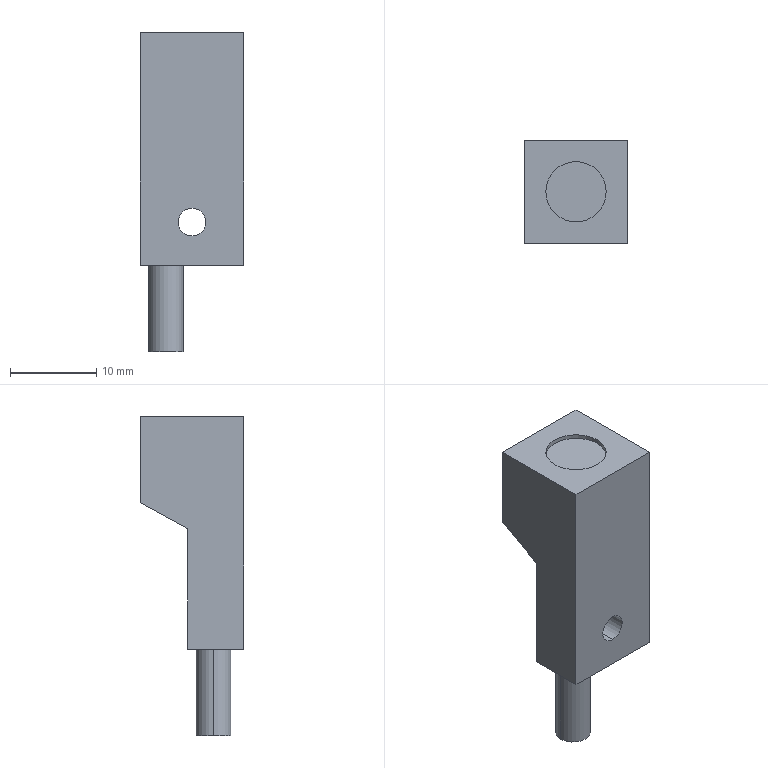Part | STEP file | 1105WWAAPS4-12M-Z-R-1-001 | 1 solid | 16 faces | box 12 x 12 x 37 mm | volume 2919 mm3 | plane 10 | cylinder 6 | commonest cylinder face diameters 3.2 x2 4 x2 7 x2
STEP:
#1=CARTESIAN_POINT('',(0.,-6.,-10.1));
#2=VERTEX_POINT('',#1);
#3=CARTESIAN_POINT('',(0.,-6.,-6.9));
#4=VERTEX_POINT('',#3);
#5=CARTESIAN_POINT('',(0.,-6.,-8.5));
#6=DIRECTION('',(0.,1.,0.));
#7=DIRECTION('',(0.,0.,1.));
#8=AXIS2_PLACEMENT_3D('',#5,#6,#7);
#9=CIRCLE('',#8,1.6);
#10=EDGE_CURVE('',#2,#4,#9,.T.);
#11=ORIENTED_EDGE('',*,*,#10,.F.);
#12=CARTESIAN_POINT('',(0.,0.5,-10.1));
#13=VERTEX_POINT('',#12);
#14=CARTESIAN_POINT('',(0.,-6.,-10.1));
#15=DIRECTION('',(0.,1.,0.));
#16=VECTOR('',#15,1000.);
#17=LINE('',#14,#16);
#18=EDGE_CURVE('',#2,#13,#17,.T.);
#19=ORIENTED_EDGE('',*,*,#18,.T.);
#20=CARTESIAN_POINT('',(0.,0.5,-6.9));
#21=VERTEX_POINT('',#20);
#22=CARTESIAN_POINT('',(0.,0.5,-8.5));
#23=DIRECTION('',(0.,1.,0.));
#24=DIRECTION('',(0.,0.,1.));
#25=AXIS2_PLACEMENT_3D('',#22,#23,#24);
#26=CIRCLE('',#25,1.6);
#27=EDGE_CURVE('',#13,#21,#26,.T.);
#28=ORIENTED_EDGE('',*,*,#27,.T.);
#29=CARTESIAN_POINT('',(0.,-6.,-6.9));
#30=DIRECTION('',(0.,1.,0.));
#31=VECTOR('',#30,1000.);
#32=LINE('',#29,#31);
#33=EDGE_CURVE('',#4,#21,#32,.T.);
#34=ORIENTED_EDGE('',*,*,#33,.F.);
#35=EDGE_LOOP('',(#11,#19,#28,#34));
#36=FACE_OUTER_BOUND('',#35,.T.);
#37=CARTESIAN_POINT('',(0.,-6.,-8.5));
#38=DIRECTION('',(0.,1.,0.));
#39=DIRECTION('',(0.,0.,1.));
#40=AXIS2_PLACEMENT_3D('',#37,#38,#39);
#41=CYLINDRICAL_SURFACE('',#40,1.6);
#42=ADVANCED_FACE('',(#36),#41,.F.);
#43=CARTESIAN_POINT('',(-5.,-2.5,-23.5));
#44=VERTEX_POINT('',#43);
#45=CARTESIAN_POINT('',(-1.,-2.5,-23.5));
#46=VERTEX_POINT('',#45);
#47=CARTESIAN_POINT('',(-3.,-2.5,-23.5));
#48=DIRECTION('',(0.,0.,-1.));
#49=DIRECTION('',(-1.,0.,0.));
#50=AXIS2_PLACEMENT_3D('',#47,#48,#49);
#51=CIRCLE('',#50,2.);
#52=EDGE_CURVE('',#44,#46,#51,.T.);
#53=ORIENTED_EDGE('',*,*,#52,.F.);
#54=CARTESIAN_POINT('',(-5.,-2.5,-13.5));
#55=VERTEX_POINT('',#54);
#56=CARTESIAN_POINT('',(-5.,-2.5,-23.5));
#57=DIRECTION('',(0.,0.,1.));
#58=VECTOR('',#57,1000.);
#59=LINE('',#56,#58);
#60=EDGE_CURVE('',#44,#55,#59,.T.);
#61=ORIENTED_EDGE('',*,*,#60,.T.);
#62=CARTESIAN_POINT('',(-1.,-2.5,-13.5));
#63=VERTEX_POINT('',#62);
#64=CARTESIAN_POINT('',(-3.,-2.5,-13.5));
#65=DIRECTION('',(0.,0.,-1.));
#66=DIRECTION('',(-1.,0.,0.));
#67=AXIS2_PLACEMENT_3D('',#64,#65,#66);
#68=CIRCLE('',#67,2.);
#69=EDGE_CURVE('',#55,#63,#68,.T.);
#70=ORIENTED_EDGE('',*,*,#69,.T.);
#71=CARTESIAN_POINT('',(-1.,-2.5,-23.5));
#72=DIRECTION('',(0.,0.,1.));
#73=VECTOR('',#72,1000.);
#74=LINE('',#71,#73);
#75=EDGE_CURVE('',#46,#63,#74,.T.);
#76=ORIENTED_EDGE('',*,*,#75,.F.);
#77=EDGE_LOOP('',(#53,#61,#70,#76));
#78=FACE_OUTER_BOUND('',#77,.T.);
#79=CARTESIAN_POINT('',(-3.,-2.5,-23.5));
#80=DIRECTION('',(0.,0.,1.));
#81=DIRECTION('',(1.,0.,0.));
#82=AXIS2_PLACEMENT_3D('',#79,#80,#81);
#83=CYLINDRICAL_SURFACE('',#82,2.);
#84=ADVANCED_FACE('',(#78),#83,.T.);
#85=CARTESIAN_POINT('',(-3.5,0.,13.));
#86=VERTEX_POINT('',#85);
#87=CARTESIAN_POINT('',(3.5,0.,13.));
#88=VERTEX_POINT('',#87);
#89=CARTESIAN_POINT('',(0.,0.,13.));
#90=DIRECTION('',(0.,0.,1.));
#91=DIRECTION('',(1.,0.,0.));
#92=AXIS2_PLACEMENT_3D('',#89,#90,#91);
#93=CIRCLE('',#92,3.5);
#94=EDGE_CURVE('',#86,#88,#93,.T.);
#95=ORIENTED_EDGE('',*,*,#94,.F.);
#96=CARTESIAN_POINT('',(-3.5,0.,13.5));
#97=VERTEX_POINT('',#96);
#98=CARTESIAN_POINT('',(-3.5,0.,13.));
#99=DIRECTION('',(0.,0.,1.));
#100=VECTOR('',#99,1000.);
#101=LINE('',#98,#100);
#102=EDGE_CURVE('',#86,#97,#101,.T.);
#103=ORIENTED_EDGE('',*,*,#102,.T.);
#104=CARTESIAN_POINT('',(3.5,0.,13.5));
#105=VERTEX_POINT('',#104);
#106=CARTESIAN_POINT('',(0.,0.,13.5));
#107=DIRECTION('',(0.,0.,1.));
#108=DIRECTION('',(1.,0.,0.));
#109=AXIS2_PLACEMENT_3D('',#106,#107,#108);
#110=CIRCLE('',#109,3.5);
#111=EDGE_CURVE('',#97,#105,#110,.T.);
#112=ORIENTED_EDGE('',*,*,#111,.T.);
#113=CARTESIAN_POINT('',(3.5,0.,13.));
#114=DIRECTION('',(0.,0.,1.));
#115=VECTOR('',#114,1000.);
#116=LINE('',#113,#115);
#117=EDGE_CURVE('',#88,#105,#116,.T.);
#118=ORIENTED_EDGE('',*,*,#117,.F.);
#119=EDGE_LOOP('',(#95,#103,#112,#118));
#120=FACE_OUTER_BOUND('',#119,.T.);
#121=CARTESIAN_POINT('',(0.,0.,13.));
#122=DIRECTION('',(0.,0.,1.));
#123=DIRECTION('',(1.,0.,0.));
#124=AXIS2_PLACEMENT_3D('',#121,#122,#123);
#125=CYLINDRICAL_SURFACE('',#124,3.5);
#126=ADVANCED_FACE('',(#120),#125,.F.);
#127=CARTESIAN_POINT('',(-6.,0.5,-13.5));
#128=VERTEX_POINT('',#127);
#129=CARTESIAN_POINT('',(-6.,-6.,-13.5));
#130=VERTEX_POINT('',#129);
#131=CARTESIAN_POINT('',(-6.,-6.,-13.5));
#132=DIRECTION('',(0.,-1.,0.));
#133=VECTOR('',#132,1000.);
#134=LINE('',#131,#133);
#135=EDGE_CURVE('',#128,#130,#134,.T.);
#136=ORIENTED_EDGE('',*,*,#135,.F.);
#137=CARTESIAN_POINT('',(6.,0.5,-13.5));
#138=VERTEX_POINT('',#137);
#139=CARTESIAN_POINT('',(6.,0.5,-13.5));
#140=DIRECTION('',(1.,0.,0.));
#141=VECTOR('',#140,1000.);
#142=LINE('',#139,#141);
#143=EDGE_CURVE('',#128,#138,#142,.T.);
#144=ORIENTED_EDGE('',*,*,#143,.T.);
#145=CARTESIAN_POINT('',(6.,-6.,-13.5));
#146=VERTEX_POINT('',#145);
#147=CARTESIAN_POINT('',(6.,-6.,-13.5));
#148=DIRECTION('',(0.,1.,0.));
#149=VECTOR('',#148,1000.);
#150=LINE('',#147,#149);
#151=EDGE_CURVE('',#146,#138,#150,.T.);
#152=ORIENTED_EDGE('',*,*,#151,.F.);
#153=CARTESIAN_POINT('',(-6.,-6.,-13.5));
#154=DIRECTION('',(1.,0.,0.));
#155=VECTOR('',#154,1000.);
#156=LINE('',#153,#155);
#157=EDGE_CURVE('',#130,#146,#156,.T.);
#158=ORIENTED_EDGE('',*,*,#157,.F.);
#159=EDGE_LOOP('',(#136,#144,#152,#158));
#160=FACE_OUTER_BOUND('',#159,.T.);
#161=CARTESIAN_POINT('',(-3.,-2.5,-13.5));
#162=DIRECTION('',(0.,0.,-1.));
#163=DIRECTION('',(-1.,0.,0.));
#164=AXIS2_PLACEMENT_3D('',#161,#162,#163);
#165=CIRCLE('',#164,2.);
#166=EDGE_CURVE('',#63,#55,#165,.T.);
#167=ORIENTED_EDGE('',*,*,#166,.F.);
#168=ORIENTED_EDGE('',*,*,#69,.F.);
#169=EDGE_LOOP('',(#167,#168));
#170=FACE_BOUND('',#169,.T.);
#171=CARTESIAN_POINT('',(6.,6.,-13.5));
#172=DIRECTION('',(0.,0.,-1.));
#173=DIRECTION('',(-1.,0.,0.));
#174=AXIS2_PLACEMENT_3D('',#171,#172,#173);
#175=PLANE('',#174);
#176=ADVANCED_FACE('',(#160,#170),#175,.T.);
#177=CARTESIAN_POINT('',(6.,6.,3.5));
#178=VERTEX_POINT('',#177);
#179=CARTESIAN_POINT('',(6.,0.5,0.5));
#180=VERTEX_POINT('',#179);
#181=CARTESIAN_POINT('',(6.,0.9554,0.7484));
#182=DIRECTION('',(0.,-0.8779,-0.4789));
#183=VECTOR('',#182,1000.);
#184=LINE('',#181,#183);
#185=EDGE_CURVE('',#178,#180,#184,.T.);
#186=ORIENTED_EDGE('',*,*,#185,.F.);
#187=CARTESIAN_POINT('',(6.,6.,13.5));
#188=VERTEX_POINT('',#187);
#189=CARTESIAN_POINT('',(6.,6.,13.5));
#190=DIRECTION('',(0.,0.,-1.));
#191=VECTOR('',#190,1000.);
#192=LINE('',#189,#191);
#193=EDGE_CURVE('',#188,#178,#192,.T.);
#194=ORIENTED_EDGE('',*,*,#193,.F.);
#195=CARTESIAN_POINT('',(6.,-6.,13.5));
#196=VERTEX_POINT('',#195);
#197=CARTESIAN_POINT('',(6.,-6.,13.5));
#198=DIRECTION('',(0.,1.,0.));
#199=VECTOR('',#198,1000.);
#200=LINE('',#197,#199);
#201=EDGE_CURVE('',#196,#188,#200,.T.);
#202=ORIENTED_EDGE('',*,*,#201,.F.);
#203=CARTESIAN_POINT('',(6.,-6.,13.5));
#204=DIRECTION('',(0.,0.,-1.));
#205=VECTOR('',#204,1000.);
#206=LINE('',#203,#205);
#207=EDGE_CURVE('',#196,#146,#206,.T.);
#208=ORIENTED_EDGE('',*,*,#207,.T.);
#209=ORIENTED_EDGE('',*,*,#151,.T.);
#210=CARTESIAN_POINT('',(6.,0.5,13.5));
#211=DIRECTION('',(0.,0.,-1.));
#212=VECTOR('',#211,1000.);
#213=LINE('',#210,#212);
#214=EDGE_CURVE('',#180,#138,#213,.T.);
#215=ORIENTED_EDGE('',*,*,#214,.F.);
#216=EDGE_LOOP('',(#186,#194,#202,#208,#209,#215));
#217=FACE_OUTER_BOUND('',#216,.T.);
#218=CARTESIAN_POINT('',(6.,-6.,13.5));
#219=DIRECTION('',(-1.,0.,0.));
#220=DIRECTION('',(0.,0.,1.));
#221=AXIS2_PLACEMENT_3D('',#218,#219,#220);
#222=PLANE('',#221);
#223=ADVANCED_FACE('',(#217),#222,.F.);
#224=CARTESIAN_POINT('',(-6.,6.,3.5));
#225=VERTEX_POINT('',#224);
#226=CARTESIAN_POINT('',(45.863,6.,3.5));
#227=DIRECTION('',(-1.,0.,0.));
#228=VECTOR('',#227,1000.);
#229=LINE('',#226,#228);
#230=EDGE_CURVE('',#178,#225,#229,.T.);
#231=ORIENTED_EDGE('',*,*,#230,.T.);
#232=CARTESIAN_POINT('',(-6.,6.,13.5));
#233=VERTEX_POINT('',#232);
#234=CARTESIAN_POINT('',(-6.,6.,13.5));
#235=DIRECTION('',(0.,0.,-1.));
#236=VECTOR('',#235,1000.);
#237=LINE('',#234,#236);
#238=EDGE_CURVE('',#233,#225,#237,.T.);
#239=ORIENTED_EDGE('',*,*,#238,.F.);
#240=CARTESIAN_POINT('',(-6.,6.,13.5));
#241=DIRECTION('',(-1.,0.,0.));
#242=VECTOR('',#241,1000.);
#243=LINE('',#240,#242);
#244=EDGE_CURVE('',#188,#233,#243,.T.);
#245=ORIENTED_EDGE('',*,*,#244,.F.);
#246=ORIENTED_EDGE('',*,*,#193,.T.);
#247=EDGE_LOOP('',(#231,#239,#245,#246));
#248=FACE_OUTER_BOUND('',#247,.T.);
#249=CARTESIAN_POINT('',(-6.,6.,13.5));
#250=DIRECTION('',(0.,-1.,0.));
#251=DIRECTION('',(0.,0.,-1.));
#252=AXIS2_PLACEMENT_3D('',#249,#250,#251);
#253=PLANE('',#252);
#254=ADVANCED_FACE('',(#248),#253,.F.);
#255=CARTESIAN_POINT('',(-6.,0.5,0.5));
#256=VERTEX_POINT('',#255);
#257=CARTESIAN_POINT('',(-6.,0.9554,0.7484));
#258=DIRECTION('',(0.,0.8779,0.4789));
#259=VECTOR('',#258,1000.);
#260=LINE('',#257,#259);
#261=EDGE_CURVE('',#256,#225,#260,.T.);
#262=ORIENTED_EDGE('',*,*,#261,.F.);
#263=CARTESIAN_POINT('',(-6.,0.5,13.5));
#264=DIRECTION('',(0.,0.,1.));
#265=VECTOR('',#264,1000.);
#266=LINE('',#263,#265);
#267=EDGE_CURVE('',#128,#256,#266,.T.);
#268=ORIENTED_EDGE('',*,*,#267,.F.);
#269=ORIENTED_EDGE('',*,*,#135,.T.);
#270=CARTESIAN_POINT('',(-6.,-6.,13.5));
#271=VERTEX_POINT('',#270);
#272=CARTESIAN_POINT('',(-6.,-6.,13.5));
#273=DIRECTION('',(0.,0.,-1.));
#274=VECTOR('',#273,1000.);
#275=LINE('',#272,#274);
#276=EDGE_CURVE('',#271,#130,#275,.T.);
#277=ORIENTED_EDGE('',*,*,#276,.F.);
#278=CARTESIAN_POINT('',(-6.,-6.,13.5));
#279=DIRECTION('',(0.,-1.,0.));
#280=VECTOR('',#279,1000.);
#281=LINE('',#278,#280);
#282=EDGE_CURVE('',#233,#271,#281,.T.);
#283=ORIENTED_EDGE('',*,*,#282,.F.);
#284=ORIENTED_EDGE('',*,*,#238,.T.);
#285=EDGE_LOOP('',(#262,#268,#269,#277,#283,#284));
#286=FACE_OUTER_BOUND('',#285,.T.);
#287=CARTESIAN_POINT('',(-6.,-6.,13.5));
#288=DIRECTION('',(1.,0.,0.));
#289=DIRECTION('',(0.,0.,-1.));
#290=AXIS2_PLACEMENT_3D('',#287,#288,#289);
#291=PLANE('',#290);
#292=ADVANCED_FACE('',(#286),#291,.F.);
#293=CARTESIAN_POINT('',(0.,-6.,-8.5));
#294=DIRECTION('',(0.,1.,0.));
#295=DIRECTION('',(0.,0.,1.));
#296=AXIS2_PLACEMENT_3D('',#293,#294,#295);
#297=CIRCLE('',#296,1.6);
#298=EDGE_CURVE('',#4,#2,#297,.T.);
#299=ORIENTED_EDGE('',*,*,#298,.T.);
#300=ORIENTED_EDGE('',*,*,#10,.T.);
#301=EDGE_LOOP('',(#299,#300));
#302=FACE_BOUND('',#301,.T.);
#303=ORIENTED_EDGE('',*,*,#157,.T.);
#304=ORIENTED_EDGE('',*,*,#207,.F.);
#305=CARTESIAN_POINT('',(-6.,-6.,13.5));
#306=DIRECTION('',(1.,0.,0.));
#307=VECTOR('',#306,1000.);
#308=LINE('',#305,#307);
#309=EDGE_CURVE('',#271,#196,#308,.T.);
#310=ORIENTED_EDGE('',*,*,#309,.F.);
#311=ORIENTED_EDGE('',*,*,#276,.T.);
#312=EDGE_LOOP('',(#303,#304,#310,#311));
#313=FACE_OUTER_BOUND('',#312,.T.);
#314=CARTESIAN_POINT('',(-6.,-6.,13.5));
#315=DIRECTION('',(0.,1.,0.));
#316=DIRECTION('',(0.,0.,1.));
#317=AXIS2_PLACEMENT_3D('',#314,#315,#316);
#318=PLANE('',#317);
#319=ADVANCED_FACE('',(#302,#313),#318,.F.);
#320=CARTESIAN_POINT('',(0.,0.,13.5));
#321=DIRECTION('',(0.,0.,1.));
#322=DIRECTION('',(1.,0.,0.));
#323=AXIS2_PLACEMENT_3D('',#320,#321,#322);
#324=CIRCLE('',#323,3.5);
#325=EDGE_CURVE('',#105,#97,#324,.T.);
#326=ORIENTED_EDGE('',*,*,#325,.F.);
#327=ORIENTED_EDGE('',*,*,#111,.F.);
#328=EDGE_LOOP('',(#326,#327));
#329=FACE_BOUND('',#328,.T.);
#330=ORIENTED_EDGE('',*,*,#201,.T.);
#331=ORIENTED_EDGE('',*,*,#244,.T.);
#332=ORIENTED_EDGE('',*,*,#282,.T.);
#333=ORIENTED_EDGE('',*,*,#309,.T.);
#334=EDGE_LOOP('',(#330,#331,#332,#333));
#335=FACE_OUTER_BOUND('',#334,.T.);
#336=CARTESIAN_POINT('',(6.,6.,13.5));
#337=DIRECTION('',(0.,0.,-1.));
#338=DIRECTION('',(-1.,0.,0.));
#339=AXIS2_PLACEMENT_3D('',#336,#337,#338);
#340=PLANE('',#339);
#341=ADVANCED_FACE('',(#329,#335),#340,.F.);
#342=ORIENTED_EDGE('',*,*,#230,.F.);
#343=ORIENTED_EDGE('',*,*,#185,.T.);
#344=CARTESIAN_POINT('',(45.863,0.5,0.5));
#345=DIRECTION('',(-1.,0.,0.));
#346=VECTOR('',#345,1000.);
#347=LINE('',#344,#346);
#348=EDGE_CURVE('',#180,#256,#347,.T.);
#349=ORIENTED_EDGE('',*,*,#348,.T.);
#350=ORIENTED_EDGE('',*,*,#261,.T.);
#351=EDGE_LOOP('',(#342,#343,#349,#350));
#352=FACE_OUTER_BOUND('',#351,.T.);
#353=CARTESIAN_POINT('',(45.863,6.,3.5));
#354=DIRECTION('',(0.,0.4789,-0.8779));
#355=DIRECTION('',(0.,0.8779,0.4789));
#356=AXIS2_PLACEMENT_3D('',#353,#354,#355);
#357=PLANE('',#356);
#358=ADVANCED_FACE('',(#352),#357,.T.);
#359=CARTESIAN_POINT('',(0.,0.5,-8.5));
#360=DIRECTION('',(0.,1.,0.));
#361=DIRECTION('',(0.,0.,1.));
#362=AXIS2_PLACEMENT_3D('',#359,#360,#361);
#363=CIRCLE('',#362,1.6);
#364=EDGE_CURVE('',#21,#13,#363,.T.);
#365=ORIENTED_EDGE('',*,*,#364,.F.);
#366=ORIENTED_EDGE('',*,*,#27,.F.);
#367=EDGE_LOOP('',(#365,#366));
#368=FACE_BOUND('',#367,.T.);
#369=ORIENTED_EDGE('',*,*,#348,.F.);
#370=ORIENTED_EDGE('',*,*,#214,.T.);
#371=ORIENTED_EDGE('',*,*,#143,.F.);
#372=ORIENTED_EDGE('',*,*,#267,.T.);
#373=EDGE_LOOP('',(#369,#370,#371,#372));
#374=FACE_OUTER_BOUND('',#373,.T.);
#375=CARTESIAN_POINT('',(45.863,0.5,0.5));
#376=DIRECTION('',(0.,1.,0.));
#377=DIRECTION('',(0.,0.,1.));
#378=AXIS2_PLACEMENT_3D('',#375,#376,#377);
#379=PLANE('',#378);
#380=ADVANCED_FACE('',(#368,#374),#379,.T.);
#381=ORIENTED_EDGE('',*,*,#102,.F.);
#382=CARTESIAN_POINT('',(0.,0.,13.));
#383=DIRECTION('',(0.,0.,1.));
#384=DIRECTION('',(1.,0.,0.));
#385=AXIS2_PLACEMENT_3D('',#382,#383,#384);
#386=CIRCLE('',#385,3.5);
#387=EDGE_CURVE('',#88,#86,#386,.T.);
#388=ORIENTED_EDGE('',*,*,#387,.F.);
#389=ORIENTED_EDGE('',*,*,#117,.T.);
#390=ORIENTED_EDGE('',*,*,#325,.T.);
#391=EDGE_LOOP('',(#381,#388,#389,#390));
#392=FACE_OUTER_BOUND('',#391,.T.);
#393=CARTESIAN_POINT('',(0.,0.,13.));
#394=DIRECTION('',(0.,0.,1.));
#395=DIRECTION('',(1.,0.,0.));
#396=AXIS2_PLACEMENT_3D('',#393,#394,#395);
#397=CYLINDRICAL_SURFACE('',#396,3.5);
#398=ADVANCED_FACE('',(#392),#397,.F.);
#399=ORIENTED_EDGE('',*,*,#387,.T.);
#400=ORIENTED_EDGE('',*,*,#94,.T.);
#401=EDGE_LOOP('',(#399,#400));
#402=FACE_OUTER_BOUND('',#401,.T.);
#403=CARTESIAN_POINT('',(0.,0.,13.));
#404=DIRECTION('',(0.,0.,1.));
#405=DIRECTION('',(1.,0.,0.));
#406=AXIS2_PLACEMENT_3D('',#403,#404,#405);
#407=PLANE('',#406);
#408=ADVANCED_FACE('',(#402),#407,.T.);
#409=ORIENTED_EDGE('',*,*,#60,.F.);
#410=CARTESIAN_POINT('',(-3.,-2.5,-23.5));
#411=DIRECTION('',(0.,0.,-1.));
#412=DIRECTION('',(-1.,0.,0.));
#413=AXIS2_PLACEMENT_3D('',#410,#411,#412);
#414=CIRCLE('',#413,2.);
#415=EDGE_CURVE('',#46,#44,#414,.T.);
#416=ORIENTED_EDGE('',*,*,#415,.F.);
#417=ORIENTED_EDGE('',*,*,#75,.T.);
#418=ORIENTED_EDGE('',*,*,#166,.T.);
#419=EDGE_LOOP('',(#409,#416,#417,#418));
#420=FACE_OUTER_BOUND('',#419,.T.);
#421=CARTESIAN_POINT('',(-3.,-2.5,-23.5));
#422=DIRECTION('',(0.,0.,1.));
#423=DIRECTION('',(1.,0.,0.));
#424=AXIS2_PLACEMENT_3D('',#421,#422,#423);
#425=CYLINDRICAL_SURFACE('',#424,2.);
#426=ADVANCED_FACE('',(#420),#425,.T.);
#427=ORIENTED_EDGE('',*,*,#415,.T.);
#428=ORIENTED_EDGE('',*,*,#52,.T.);
#429=EDGE_LOOP('',(#427,#428));
#430=FACE_OUTER_BOUND('',#429,.T.);
#431=CARTESIAN_POINT('',(-3.,-2.5,-23.5));
#432=DIRECTION('',(0.,0.,-1.));
#433=DIRECTION('',(-1.,0.,0.));
#434=AXIS2_PLACEMENT_3D('',#431,#432,#433);
#435=PLANE('',#434);
#436=ADVANCED_FACE('',(#430),#435,.T.);
#437=ORIENTED_EDGE('',*,*,#18,.F.);
#438=ORIENTED_EDGE('',*,*,#298,.F.);
#439=ORIENTED_EDGE('',*,*,#33,.T.);
#440=ORIENTED_EDGE('',*,*,#364,.T.);
#441=EDGE_LOOP('',(#437,#438,#439,#440));
#442=FACE_OUTER_BOUND('',#441,.T.);
#443=CARTESIAN_POINT('',(0.,-6.,-8.5));
#444=DIRECTION('',(0.,1.,0.));
#445=DIRECTION('',(0.,0.,1.));
#446=AXIS2_PLACEMENT_3D('',#443,#444,#445);
#447=CYLINDRICAL_SURFACE('',#446,1.6);
#448=ADVANCED_FACE('',(#442),#447,.F.);
#449=CLOSED_SHELL('',(#42,#84,#126,#176,#223,#254,#292,#319,#341,#358,#380,#398,#408,#426,#436,#448));
#450=MANIFOLD_SOLID_BREP('',#449);
#451=CARTESIAN_POINT('',(0.,0.,0.));
#452=DIRECTION('',(0.,0.,1.));
#453=DIRECTION('',(1.,0.,0.));
#454=AXIS2_PLACEMENT_3D('',#451,#452,#453);
#455=(LENGTH_UNIT()NAMED_UNIT(*)SI_UNIT(.MILLI.,.METRE.));
#456=UNCERTAINTY_MEASURE_WITH_UNIT(LENGTH_MEASURE(0.00001),#455,'','');
#457=(NAMED_UNIT(*)PLANE_ANGLE_UNIT()SI_UNIT($,.RADIAN.));
#458=(NAMED_UNIT(*)SI_UNIT($,.STERADIAN.)SOLID_ANGLE_UNIT());
#459=(GEOMETRIC_REPRESENTATION_CONTEXT(3)GLOBAL_UNCERTAINTY_ASSIGNED_CONTEXT((#456))GLOBAL_UNIT_ASSIGNED_CONTEXT((#455,#457,#458))REPRESENTATION_CONTEXT('',''));
#460=ADVANCED_BREP_SHAPE_REPRESENTATION('',(#450,#454),#459);